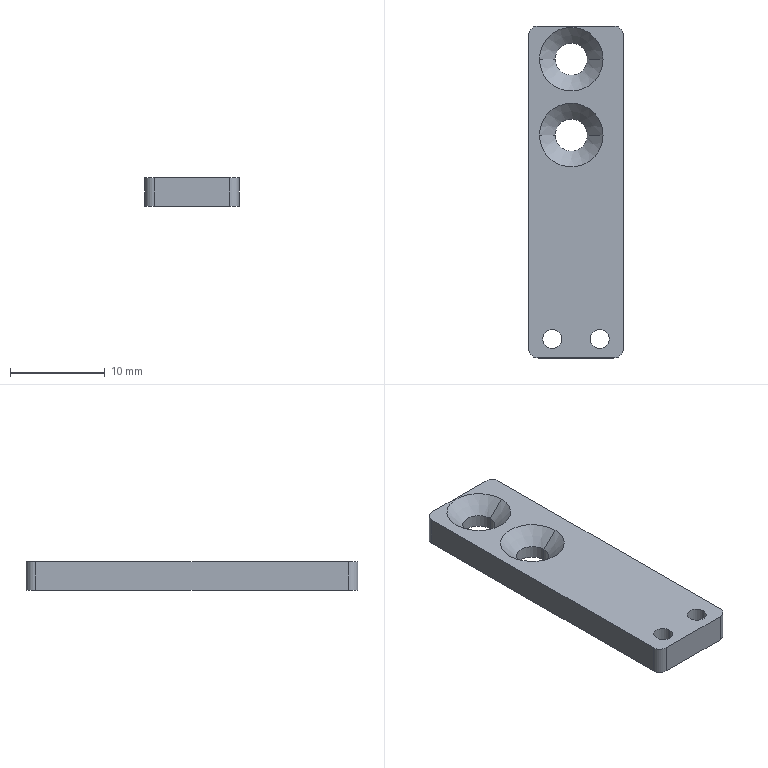Part | STEP file | 11-FG-B08211 | 1 solid | 22 faces | box 10 x 35 x 3 mm | volume 935.086 mm3 | cylinder 12 | plane 6 | cone 4 | commonest cylinder face diameters 2 x8 3.4 x4
STEP:
#1=CARTESIAN_POINT('',(3.5,-15.5,0.));
#2=VERTEX_POINT('',#1);
#3=CARTESIAN_POINT('',(1.5,-15.5,0.));
#4=VERTEX_POINT('',#3);
#5=CARTESIAN_POINT('',(2.5,-15.5,0.));
#6=DIRECTION('',(0.,0.,-1.));
#7=DIRECTION('',(1.,0.,0.));
#8=AXIS2_PLACEMENT_3D('',#5,#6,#7);
#9=CIRCLE('',#8,1.);
#10=EDGE_CURVE('',#2,#4,#9,.T.);
#11=ORIENTED_EDGE('',*,*,#10,.T.);
#12=CARTESIAN_POINT('',(1.5,-15.5,3.));
#13=VERTEX_POINT('',#12);
#14=CARTESIAN_POINT('',(1.5,-15.5,-7.));
#15=DIRECTION('',(0.,0.,1.));
#16=VECTOR('',#15,1000.);
#17=LINE('',#14,#16);
#18=EDGE_CURVE('',#4,#13,#17,.T.);
#19=ORIENTED_EDGE('',*,*,#18,.T.);
#20=CARTESIAN_POINT('',(3.5,-15.5,3.));
#21=VERTEX_POINT('',#20);
#22=CARTESIAN_POINT('',(2.5,-15.5,3.));
#23=DIRECTION('',(0.,0.,-1.));
#24=DIRECTION('',(-1.,0.,0.));
#25=AXIS2_PLACEMENT_3D('',#22,#23,#24);
#26=CIRCLE('',#25,1.);
#27=EDGE_CURVE('',#21,#13,#26,.T.);
#28=ORIENTED_EDGE('',*,*,#27,.F.);
#29=CARTESIAN_POINT('',(3.5,-15.5,-7.));
#30=DIRECTION('',(0.,0.,1.));
#31=VECTOR('',#30,1000.);
#32=LINE('',#29,#31);
#33=EDGE_CURVE('',#2,#21,#32,.T.);
#34=ORIENTED_EDGE('',*,*,#33,.F.);
#35=EDGE_LOOP('',(#11,#19,#28,#34));
#36=FACE_OUTER_BOUND('',#35,.T.);
#37=CARTESIAN_POINT('',(2.5,-15.5,-7.));
#38=DIRECTION('',(0.,0.,1.));
#39=DIRECTION('',(1.,0.,0.));
#40=AXIS2_PLACEMENT_3D('',#37,#38,#39);
#41=CYLINDRICAL_SURFACE('',#40,1.);
#42=ADVANCED_FACE('',(#36),#41,.F.);
#43=CARTESIAN_POINT('',(-3.5,-15.5,0.));
#44=VERTEX_POINT('',#43);
#45=CARTESIAN_POINT('',(-1.5,-15.5,0.));
#46=VERTEX_POINT('',#45);
#47=CARTESIAN_POINT('',(-2.5,-15.5,0.));
#48=DIRECTION('',(0.,0.,1.));
#49=DIRECTION('',(1.,0.,0.));
#50=AXIS2_PLACEMENT_3D('',#47,#48,#49);
#51=CIRCLE('',#50,1.);
#52=EDGE_CURVE('',#44,#46,#51,.T.);
#53=ORIENTED_EDGE('',*,*,#52,.F.);
#54=CARTESIAN_POINT('',(-3.5,-15.5,3.));
#55=VERTEX_POINT('',#54);
#56=CARTESIAN_POINT('',(-3.5,-15.5,-7.));
#57=DIRECTION('',(0.,0.,1.));
#58=VECTOR('',#57,1000.);
#59=LINE('',#56,#58);
#60=EDGE_CURVE('',#44,#55,#59,.T.);
#61=ORIENTED_EDGE('',*,*,#60,.T.);
#62=CARTESIAN_POINT('',(-1.5,-15.5,3.));
#63=VERTEX_POINT('',#62);
#64=CARTESIAN_POINT('',(-2.5,-15.5,3.));
#65=DIRECTION('',(0.,0.,1.));
#66=DIRECTION('',(1.,0.,0.));
#67=AXIS2_PLACEMENT_3D('',#64,#65,#66);
#68=CIRCLE('',#67,1.);
#69=EDGE_CURVE('',#55,#63,#68,.T.);
#70=ORIENTED_EDGE('',*,*,#69,.T.);
#71=CARTESIAN_POINT('',(-1.5,-15.5,-7.));
#72=DIRECTION('',(0.,0.,1.));
#73=VECTOR('',#72,1000.);
#74=LINE('',#71,#73);
#75=EDGE_CURVE('',#46,#63,#74,.T.);
#76=ORIENTED_EDGE('',*,*,#75,.F.);
#77=EDGE_LOOP('',(#53,#61,#70,#76));
#78=FACE_OUTER_BOUND('',#77,.T.);
#79=CARTESIAN_POINT('',(-2.5,-15.5,-7.));
#80=DIRECTION('',(0.,0.,1.));
#81=DIRECTION('',(1.,0.,0.));
#82=AXIS2_PLACEMENT_3D('',#79,#80,#81);
#83=CYLINDRICAL_SURFACE('',#82,1.);
#84=ADVANCED_FACE('',(#78),#83,.F.);
#85=CARTESIAN_POINT('',(-2.2,14.,1.34));
#86=VERTEX_POINT('',#85);
#87=CARTESIAN_POINT('',(1.2,14.,1.34));
#88=VERTEX_POINT('',#87);
#89=CARTESIAN_POINT('',(-0.5,14.,1.34));
#90=DIRECTION('',(0.,0.,1.));
#91=DIRECTION('',(1.,0.,0.));
#92=AXIS2_PLACEMENT_3D('',#89,#90,#91);
#93=CIRCLE('',#92,1.7);
#94=EDGE_CURVE('',#86,#88,#93,.T.);
#95=ORIENTED_EDGE('',*,*,#94,.F.);
#96=CARTESIAN_POINT('',(-3.86,14.,3.));
#97=VERTEX_POINT('',#96);
#98=CARTESIAN_POINT('',(-3.86,14.,3.));
#99=DIRECTION('',(-0.7071,0.,0.7071));
#100=VECTOR('',#99,1000.);
#101=LINE('',#98,#100);
#102=EDGE_CURVE('',#86,#97,#101,.T.);
#103=ORIENTED_EDGE('',*,*,#102,.T.);
#104=CARTESIAN_POINT('',(2.86,14.,3.));
#105=VERTEX_POINT('',#104);
#106=CARTESIAN_POINT('',(-0.5,14.,3.));
#107=DIRECTION('',(0.,0.,1.));
#108=DIRECTION('',(1.,0.,0.));
#109=AXIS2_PLACEMENT_3D('',#106,#107,#108);
#110=CIRCLE('',#109,3.36);
#111=EDGE_CURVE('',#97,#105,#110,.T.);
#112=ORIENTED_EDGE('',*,*,#111,.T.);
#113=CARTESIAN_POINT('',(2.86,14.,3.));
#114=DIRECTION('',(0.7071,0.,0.7071));
#115=VECTOR('',#114,1000.);
#116=LINE('',#113,#115);
#117=EDGE_CURVE('',#88,#105,#116,.T.);
#118=ORIENTED_EDGE('',*,*,#117,.F.);
#119=EDGE_LOOP('',(#95,#103,#112,#118));
#120=FACE_OUTER_BOUND('',#119,.T.);
#121=CARTESIAN_POINT('',(-0.5,14.,3.));
#122=DIRECTION('',(0.,0.,1.));
#123=DIRECTION('',(1.,0.,0.));
#124=AXIS2_PLACEMENT_3D('',#121,#122,#123);
#125=CONICAL_SURFACE('',#124,3.36,0.7854);
#126=ADVANCED_FACE('',(#120),#125,.F.);
#127=CARTESIAN_POINT('',(-2.2,14.,0.));
#128=VERTEX_POINT('',#127);
#129=CARTESIAN_POINT('',(1.2,14.,0.));
#130=VERTEX_POINT('',#129);
#131=CARTESIAN_POINT('',(-0.5,14.,0.));
#132=DIRECTION('',(0.,0.,1.));
#133=DIRECTION('',(1.,0.,0.));
#134=AXIS2_PLACEMENT_3D('',#131,#132,#133);
#135=CIRCLE('',#134,1.7);
#136=EDGE_CURVE('',#128,#130,#135,.T.);
#137=ORIENTED_EDGE('',*,*,#136,.F.);
#138=CARTESIAN_POINT('',(-2.2,14.,3.));
#139=DIRECTION('',(0.,0.,1.));
#140=VECTOR('',#139,1000.);
#141=LINE('',#138,#140);
#142=EDGE_CURVE('',#128,#86,#141,.T.);
#143=ORIENTED_EDGE('',*,*,#142,.T.);
#144=ORIENTED_EDGE('',*,*,#94,.T.);
#145=CARTESIAN_POINT('',(1.2,14.,3.));
#146=DIRECTION('',(0.,0.,1.));
#147=VECTOR('',#146,1000.);
#148=LINE('',#145,#147);
#149=EDGE_CURVE('',#130,#88,#148,.T.);
#150=ORIENTED_EDGE('',*,*,#149,.F.);
#151=EDGE_LOOP('',(#137,#143,#144,#150));
#152=FACE_OUTER_BOUND('',#151,.T.);
#153=CARTESIAN_POINT('',(-0.5,14.,3.));
#154=DIRECTION('',(0.,0.,1.));
#155=DIRECTION('',(1.,0.,0.));
#156=AXIS2_PLACEMENT_3D('',#153,#154,#155);
#157=CYLINDRICAL_SURFACE('',#156,1.7);
#158=ADVANCED_FACE('',(#152),#157,.F.);
#159=CARTESIAN_POINT('',(-2.2,6.,1.34));
#160=VERTEX_POINT('',#159);
#161=CARTESIAN_POINT('',(1.2,6.,1.34));
#162=VERTEX_POINT('',#161);
#163=CARTESIAN_POINT('',(-0.5,6.,1.34));
#164=DIRECTION('',(0.,0.,1.));
#165=DIRECTION('',(1.,0.,0.));
#166=AXIS2_PLACEMENT_3D('',#163,#164,#165);
#167=CIRCLE('',#166,1.7);
#168=EDGE_CURVE('',#160,#162,#167,.T.);
#169=ORIENTED_EDGE('',*,*,#168,.F.);
#170=CARTESIAN_POINT('',(-3.86,6.,3.));
#171=VERTEX_POINT('',#170);
#172=CARTESIAN_POINT('',(-3.86,6.,3.));
#173=DIRECTION('',(-0.7071,0.,0.7071));
#174=VECTOR('',#173,1000.);
#175=LINE('',#172,#174);
#176=EDGE_CURVE('',#160,#171,#175,.T.);
#177=ORIENTED_EDGE('',*,*,#176,.T.);
#178=CARTESIAN_POINT('',(2.86,6.,3.));
#179=VERTEX_POINT('',#178);
#180=CARTESIAN_POINT('',(-0.5,6.,3.));
#181=DIRECTION('',(0.,0.,1.));
#182=DIRECTION('',(1.,0.,0.));
#183=AXIS2_PLACEMENT_3D('',#180,#181,#182);
#184=CIRCLE('',#183,3.36);
#185=EDGE_CURVE('',#171,#179,#184,.T.);
#186=ORIENTED_EDGE('',*,*,#185,.T.);
#187=CARTESIAN_POINT('',(2.86,6.,3.));
#188=DIRECTION('',(0.7071,0.,0.7071));
#189=VECTOR('',#188,1000.);
#190=LINE('',#187,#189);
#191=EDGE_CURVE('',#162,#179,#190,.T.);
#192=ORIENTED_EDGE('',*,*,#191,.F.);
#193=EDGE_LOOP('',(#169,#177,#186,#192));
#194=FACE_OUTER_BOUND('',#193,.T.);
#195=CARTESIAN_POINT('',(-0.5,6.,3.));
#196=DIRECTION('',(0.,0.,1.));
#197=DIRECTION('',(1.,0.,0.));
#198=AXIS2_PLACEMENT_3D('',#195,#196,#197);
#199=CONICAL_SURFACE('',#198,3.36,0.7854);
#200=ADVANCED_FACE('',(#194),#199,.F.);
#201=CARTESIAN_POINT('',(-2.2,6.,0.));
#202=VERTEX_POINT('',#201);
#203=CARTESIAN_POINT('',(1.2,6.,0.));
#204=VERTEX_POINT('',#203);
#205=CARTESIAN_POINT('',(-0.5,6.,0.));
#206=DIRECTION('',(0.,0.,1.));
#207=DIRECTION('',(1.,0.,0.));
#208=AXIS2_PLACEMENT_3D('',#205,#206,#207);
#209=CIRCLE('',#208,1.7);
#210=EDGE_CURVE('',#202,#204,#209,.T.);
#211=ORIENTED_EDGE('',*,*,#210,.F.);
#212=CARTESIAN_POINT('',(-2.2,6.,3.));
#213=DIRECTION('',(0.,0.,1.));
#214=VECTOR('',#213,1000.);
#215=LINE('',#212,#214);
#216=EDGE_CURVE('',#202,#160,#215,.T.);
#217=ORIENTED_EDGE('',*,*,#216,.T.);
#218=ORIENTED_EDGE('',*,*,#168,.T.);
#219=CARTESIAN_POINT('',(1.2,6.,3.));
#220=DIRECTION('',(0.,0.,1.));
#221=VECTOR('',#220,1000.);
#222=LINE('',#219,#221);
#223=EDGE_CURVE('',#204,#162,#222,.T.);
#224=ORIENTED_EDGE('',*,*,#223,.F.);
#225=EDGE_LOOP('',(#211,#217,#218,#224));
#226=FACE_OUTER_BOUND('',#225,.T.);
#227=CARTESIAN_POINT('',(-0.5,6.,3.));
#228=DIRECTION('',(0.,0.,1.));
#229=DIRECTION('',(1.,0.,0.));
#230=AXIS2_PLACEMENT_3D('',#227,#228,#229);
#231=CYLINDRICAL_SURFACE('',#230,1.7);
#232=ADVANCED_FACE('',(#226),#231,.F.);
#233=CARTESIAN_POINT('',(5.,-16.5,0.));
#234=VERTEX_POINT('',#233);
#235=CARTESIAN_POINT('',(5.,16.5,0.));
#236=VERTEX_POINT('',#235);
#237=CARTESIAN_POINT('',(5.,17.5,0.));
#238=DIRECTION('',(0.,1.,0.));
#239=VECTOR('',#238,1000.);
#240=LINE('',#237,#239);
#241=EDGE_CURVE('',#234,#236,#240,.T.);
#242=ORIENTED_EDGE('',*,*,#241,.T.);
#243=CARTESIAN_POINT('',(5.,16.5,3.));
#244=VERTEX_POINT('',#243);
#245=CARTESIAN_POINT('',(5.,16.5,3.));
#246=DIRECTION('',(0.,0.,1.));
#247=VECTOR('',#246,1000.);
#248=LINE('',#245,#247);
#249=EDGE_CURVE('',#236,#244,#248,.T.);
#250=ORIENTED_EDGE('',*,*,#249,.T.);
#251=CARTESIAN_POINT('',(5.,-16.5,3.));
#252=VERTEX_POINT('',#251);
#253=CARTESIAN_POINT('',(5.,17.5,3.));
#254=DIRECTION('',(0.,1.,0.));
#255=VECTOR('',#254,1000.);
#256=LINE('',#253,#255);
#257=EDGE_CURVE('',#252,#244,#256,.T.);
#258=ORIENTED_EDGE('',*,*,#257,.F.);
#259=CARTESIAN_POINT('',(5.,-16.5,3.));
#260=DIRECTION('',(0.,0.,-1.));
#261=VECTOR('',#260,1000.);
#262=LINE('',#259,#261);
#263=EDGE_CURVE('',#252,#234,#262,.T.);
#264=ORIENTED_EDGE('',*,*,#263,.T.);
#265=EDGE_LOOP('',(#242,#250,#258,#264));
#266=FACE_OUTER_BOUND('',#265,.T.);
#267=CARTESIAN_POINT('',(5.,17.5,3.));
#268=DIRECTION('',(-1.,0.,0.));
#269=DIRECTION('',(0.,-1.,0.));
#270=AXIS2_PLACEMENT_3D('',#267,#268,#269);
#271=PLANE('',#270);
#272=ADVANCED_FACE('',(#266),#271,.F.);
#273=CARTESIAN_POINT('',(4.,17.5,3.));
#274=VERTEX_POINT('',#273);
#275=CARTESIAN_POINT('',(-4.,17.5,3.));
#276=VERTEX_POINT('',#275);
#277=CARTESIAN_POINT('',(-5.,17.5,3.));
#278=DIRECTION('',(-1.,0.,0.));
#279=VECTOR('',#278,1000.);
#280=LINE('',#277,#279);
#281=EDGE_CURVE('',#274,#276,#280,.T.);
#282=ORIENTED_EDGE('',*,*,#281,.F.);
#283=CARTESIAN_POINT('',(4.,17.5,0.));
#284=VERTEX_POINT('',#283);
#285=CARTESIAN_POINT('',(4.,17.5,3.));
#286=DIRECTION('',(0.,0.,-1.));
#287=VECTOR('',#286,1000.);
#288=LINE('',#285,#287);
#289=EDGE_CURVE('',#274,#284,#288,.T.);
#290=ORIENTED_EDGE('',*,*,#289,.T.);
#291=CARTESIAN_POINT('',(-4.,17.5,0.));
#292=VERTEX_POINT('',#291);
#293=CARTESIAN_POINT('',(-5.,17.5,0.));
#294=DIRECTION('',(-1.,0.,0.));
#295=VECTOR('',#294,1000.);
#296=LINE('',#293,#295);
#297=EDGE_CURVE('',#284,#292,#296,.T.);
#298=ORIENTED_EDGE('',*,*,#297,.T.);
#299=CARTESIAN_POINT('',(-4.,17.5,3.));
#300=DIRECTION('',(0.,0.,1.));
#301=VECTOR('',#300,1000.);
#302=LINE('',#299,#301);
#303=EDGE_CURVE('',#292,#276,#302,.T.);
#304=ORIENTED_EDGE('',*,*,#303,.T.);
#305=EDGE_LOOP('',(#282,#290,#298,#304));
#306=FACE_OUTER_BOUND('',#305,.T.);
#307=CARTESIAN_POINT('',(-5.,17.5,3.));
#308=DIRECTION('',(0.,-1.,0.));
#309=DIRECTION('',(0.,0.,-1.));
#310=AXIS2_PLACEMENT_3D('',#307,#308,#309);
#311=PLANE('',#310);
#312=ADVANCED_FACE('',(#306),#311,.F.);
#313=CARTESIAN_POINT('',(-5.,16.5,3.));
#314=VERTEX_POINT('',#313);
#315=CARTESIAN_POINT('',(-5.,-16.5,3.));
#316=VERTEX_POINT('',#315);
#317=CARTESIAN_POINT('',(-5.,17.5,3.));
#318=DIRECTION('',(0.,-1.,0.));
#319=VECTOR('',#318,1000.);
#320=LINE('',#317,#319);
#321=EDGE_CURVE('',#314,#316,#320,.T.);
#322=ORIENTED_EDGE('',*,*,#321,.F.);
#323=CARTESIAN_POINT('',(-5.,16.5,0.));
#324=VERTEX_POINT('',#323);
#325=CARTESIAN_POINT('',(-5.,16.5,3.));
#326=DIRECTION('',(0.,0.,-1.));
#327=VECTOR('',#326,1000.);
#328=LINE('',#325,#327);
#329=EDGE_CURVE('',#314,#324,#328,.T.);
#330=ORIENTED_EDGE('',*,*,#329,.T.);
#331=CARTESIAN_POINT('',(-5.,-16.5,0.));
#332=VERTEX_POINT('',#331);
#333=CARTESIAN_POINT('',(-5.,17.5,0.));
#334=DIRECTION('',(0.,-1.,0.));
#335=VECTOR('',#334,1000.);
#336=LINE('',#333,#335);
#337=EDGE_CURVE('',#324,#332,#336,.T.);
#338=ORIENTED_EDGE('',*,*,#337,.T.);
#339=CARTESIAN_POINT('',(-5.,-16.5,3.));
#340=DIRECTION('',(0.,0.,1.));
#341=VECTOR('',#340,1000.);
#342=LINE('',#339,#341);
#343=EDGE_CURVE('',#332,#316,#342,.T.);
#344=ORIENTED_EDGE('',*,*,#343,.T.);
#345=EDGE_LOOP('',(#322,#330,#338,#344));
#346=FACE_OUTER_BOUND('',#345,.T.);
#347=CARTESIAN_POINT('',(-5.,17.5,3.));
#348=DIRECTION('',(1.,0.,0.));
#349=DIRECTION('',(0.,1.,0.));
#350=AXIS2_PLACEMENT_3D('',#347,#348,#349);
#351=PLANE('',#350);
#352=ADVANCED_FACE('',(#346),#351,.F.);
#353=CARTESIAN_POINT('',(-4.,-17.5,0.));
#354=VERTEX_POINT('',#353);
#355=CARTESIAN_POINT('',(4.,-17.5,0.));
#356=VERTEX_POINT('',#355);
#357=CARTESIAN_POINT('',(-5.,-17.5,0.));
#358=DIRECTION('',(1.,0.,0.));
#359=VECTOR('',#358,1000.);
#360=LINE('',#357,#359);
#361=EDGE_CURVE('',#354,#356,#360,.T.);
#362=ORIENTED_EDGE('',*,*,#361,.T.);
#363=CARTESIAN_POINT('',(4.,-17.5,3.));
#364=VERTEX_POINT('',#363);
#365=CARTESIAN_POINT('',(4.,-17.5,3.));
#366=DIRECTION('',(0.,0.,1.));
#367=VECTOR('',#366,1000.);
#368=LINE('',#365,#367);
#369=EDGE_CURVE('',#356,#364,#368,.T.);
#370=ORIENTED_EDGE('',*,*,#369,.T.);
#371=CARTESIAN_POINT('',(-4.,-17.5,3.));
#372=VERTEX_POINT('',#371);
#373=CARTESIAN_POINT('',(-5.,-17.5,3.));
#374=DIRECTION('',(1.,0.,0.));
#375=VECTOR('',#374,1000.);
#376=LINE('',#373,#375);
#377=EDGE_CURVE('',#372,#364,#376,.T.);
#378=ORIENTED_EDGE('',*,*,#377,.F.);
#379=CARTESIAN_POINT('',(-4.,-17.5,3.));
#380=DIRECTION('',(0.,0.,-1.));
#381=VECTOR('',#380,1000.);
#382=LINE('',#379,#381);
#383=EDGE_CURVE('',#372,#354,#382,.T.);
#384=ORIENTED_EDGE('',*,*,#383,.T.);
#385=EDGE_LOOP('',(#362,#370,#378,#384));
#386=FACE_OUTER_BOUND('',#385,.T.);
#387=CARTESIAN_POINT('',(-5.,-17.5,3.));
#388=DIRECTION('',(0.,1.,0.));
#389=DIRECTION('',(0.,0.,1.));
#390=AXIS2_PLACEMENT_3D('',#387,#388,#389);
#391=PLANE('',#390);
#392=ADVANCED_FACE('',(#386),#391,.F.);
#393=ORIENTED_EDGE('',*,*,#27,.T.);
#394=CARTESIAN_POINT('',(2.5,-15.5,3.));
#395=DIRECTION('',(0.,0.,-1.));
#396=DIRECTION('',(-1.,0.,0.));
#397=AXIS2_PLACEMENT_3D('',#394,#395,#396);
#398=CIRCLE('',#397,1.);
#399=EDGE_CURVE('',#13,#21,#398,.T.);
#400=ORIENTED_EDGE('',*,*,#399,.T.);
#401=EDGE_LOOP('',(#393,#400));
#402=FACE_BOUND('',#401,.T.);
#403=CARTESIAN_POINT('',(-2.5,-15.5,3.));
#404=DIRECTION('',(0.,0.,1.));
#405=DIRECTION('',(1.,0.,0.));
#406=AXIS2_PLACEMENT_3D('',#403,#404,#405);
#407=CIRCLE('',#406,1.);
#408=EDGE_CURVE('',#63,#55,#407,.T.);
#409=ORIENTED_EDGE('',*,*,#408,.F.);
#410=ORIENTED_EDGE('',*,*,#69,.F.);
#411=EDGE_LOOP('',(#409,#410));
#412=FACE_BOUND('',#411,.T.);
#413=CARTESIAN_POINT('',(-0.5,14.,3.));
#414=DIRECTION('',(0.,0.,1.));
#415=DIRECTION('',(1.,0.,0.));
#416=AXIS2_PLACEMENT_3D('',#413,#414,#415);
#417=CIRCLE('',#416,3.36);
#418=EDGE_CURVE('',#105,#97,#417,.T.);
#419=ORIENTED_EDGE('',*,*,#418,.F.);
#420=ORIENTED_EDGE('',*,*,#111,.F.);
#421=EDGE_LOOP('',(#419,#420));
#422=FACE_BOUND('',#421,.T.);
#423=CARTESIAN_POINT('',(-0.5,6.,3.));
#424=DIRECTION('',(0.,0.,1.));
#425=DIRECTION('',(1.,0.,0.));
#426=AXIS2_PLACEMENT_3D('',#423,#424,#425);
#427=CIRCLE('',#426,3.36);
#428=EDGE_CURVE('',#179,#171,#427,.T.);
#429=ORIENTED_EDGE('',*,*,#428,.F.);
#430=ORIENTED_EDGE('',*,*,#185,.F.);
#431=EDGE_LOOP('',(#429,#430));
#432=FACE_BOUND('',#431,.T.);
#433=ORIENTED_EDGE('',*,*,#257,.T.);
#434=CARTESIAN_POINT('',(4.,16.5,3.));
#435=DIRECTION('',(0.,0.,1.));
#436=DIRECTION('',(1.,0.,0.));
#437=AXIS2_PLACEMENT_3D('',#434,#435,#436);
#438=CIRCLE('',#437,1.);
#439=EDGE_CURVE('',#244,#274,#438,.T.);
#440=ORIENTED_EDGE('',*,*,#439,.T.);
#441=ORIENTED_EDGE('',*,*,#281,.T.);
#442=CARTESIAN_POINT('',(-4.,16.5,3.));
#443=DIRECTION('',(0.,0.,1.));
#444=DIRECTION('',(1.,0.,0.));
#445=AXIS2_PLACEMENT_3D('',#442,#443,#444);
#446=CIRCLE('',#445,1.);
#447=EDGE_CURVE('',#276,#314,#446,.T.);
#448=ORIENTED_EDGE('',*,*,#447,.T.);
#449=ORIENTED_EDGE('',*,*,#321,.T.);
#450=CARTESIAN_POINT('',(-4.,-16.5,3.));
#451=DIRECTION('',(0.,0.,1.));
#452=DIRECTION('',(1.,0.,0.));
#453=AXIS2_PLACEMENT_3D('',#450,#451,#452);
#454=CIRCLE('',#453,1.);
#455=EDGE_CURVE('',#316,#372,#454,.T.);
#456=ORIENTED_EDGE('',*,*,#455,.T.);
#457=ORIENTED_EDGE('',*,*,#377,.T.);
#458=CARTESIAN_POINT('',(4.,-16.5,3.));
#459=DIRECTION('',(0.,0.,1.));
#460=DIRECTION('',(1.,0.,0.));
#461=AXIS2_PLACEMENT_3D('',#458,#459,#460);
#462=CIRCLE('',#461,1.);
#463=EDGE_CURVE('',#364,#252,#462,.T.);
#464=ORIENTED_EDGE('',*,*,#463,.T.);
#465=EDGE_LOOP('',(#433,#440,#441,#448,#449,#456,#457,#464));
#466=FACE_OUTER_BOUND('',#465,.T.);
#467=CARTESIAN_POINT('',(0.,0.,3.));
#468=DIRECTION('',(0.,0.,1.));
#469=DIRECTION('',(1.,0.,0.));
#470=AXIS2_PLACEMENT_3D('',#467,#468,#469);
#471=PLANE('',#470);
#472=ADVANCED_FACE('',(#402,#412,#422,#432,#466),#471,.T.);
#473=ORIENTED_EDGE('',*,*,#10,.F.);
#474=CARTESIAN_POINT('',(2.5,-15.5,0.));
#475=DIRECTION('',(0.,0.,-1.));
#476=DIRECTION('',(1.,0.,0.));
#477=AXIS2_PLACEMENT_3D('',#474,#475,#476);
#478=CIRCLE('',#477,1.);
#479=EDGE_CURVE('',#4,#2,#478,.T.);
#480=ORIENTED_EDGE('',*,*,#479,.F.);
#481=EDGE_LOOP('',(#473,#480));
#482=FACE_BOUND('',#481,.T.);
#483=CARTESIAN_POINT('',(-2.5,-15.5,0.));
#484=DIRECTION('',(0.,0.,1.));
#485=DIRECTION('',(1.,0.,0.));
#486=AXIS2_PLACEMENT_3D('',#483,#484,#485);
#487=CIRCLE('',#486,1.);
#488=EDGE_CURVE('',#46,#44,#487,.T.);
#489=ORIENTED_EDGE('',*,*,#488,.T.);
#490=ORIENTED_EDGE('',*,*,#52,.T.);
#491=EDGE_LOOP('',(#489,#490));
#492=FACE_BOUND('',#491,.T.);
#493=CARTESIAN_POINT('',(-0.5,14.,0.));
#494=DIRECTION('',(0.,0.,1.));
#495=DIRECTION('',(1.,0.,0.));
#496=AXIS2_PLACEMENT_3D('',#493,#494,#495);
#497=CIRCLE('',#496,1.7);
#498=EDGE_CURVE('',#130,#128,#497,.T.);
#499=ORIENTED_EDGE('',*,*,#498,.T.);
#500=ORIENTED_EDGE('',*,*,#136,.T.);
#501=EDGE_LOOP('',(#499,#500));
#502=FACE_BOUND('',#501,.T.);
#503=CARTESIAN_POINT('',(-0.5,6.,0.));
#504=DIRECTION('',(0.,0.,1.));
#505=DIRECTION('',(1.,0.,0.));
#506=AXIS2_PLACEMENT_3D('',#503,#504,#505);
#507=CIRCLE('',#506,1.7);
#508=EDGE_CURVE('',#204,#202,#507,.T.);
#509=ORIENTED_EDGE('',*,*,#508,.T.);
#510=ORIENTED_EDGE('',*,*,#210,.T.);
#511=EDGE_LOOP('',(#509,#510));
#512=FACE_BOUND('',#511,.T.);
#513=ORIENTED_EDGE('',*,*,#297,.F.);
#514=CARTESIAN_POINT('',(4.,16.5,0.));
#515=DIRECTION('',(0.,0.,-1.));
#516=DIRECTION('',(1.,0.,0.));
#517=AXIS2_PLACEMENT_3D('',#514,#515,#516);
#518=CIRCLE('',#517,1.);
#519=EDGE_CURVE('',#284,#236,#518,.T.);
#520=ORIENTED_EDGE('',*,*,#519,.T.);
#521=ORIENTED_EDGE('',*,*,#241,.F.);
#522=CARTESIAN_POINT('',(4.,-16.5,0.));
#523=DIRECTION('',(0.,0.,-1.));
#524=DIRECTION('',(1.,0.,0.));
#525=AXIS2_PLACEMENT_3D('',#522,#523,#524);
#526=CIRCLE('',#525,1.);
#527=EDGE_CURVE('',#234,#356,#526,.T.);
#528=ORIENTED_EDGE('',*,*,#527,.T.);
#529=ORIENTED_EDGE('',*,*,#361,.F.);
#530=CARTESIAN_POINT('',(-4.,-16.5,0.));
#531=DIRECTION('',(0.,0.,-1.));
#532=DIRECTION('',(1.,0.,0.));
#533=AXIS2_PLACEMENT_3D('',#530,#531,#532);
#534=CIRCLE('',#533,1.);
#535=EDGE_CURVE('',#354,#332,#534,.T.);
#536=ORIENTED_EDGE('',*,*,#535,.T.);
#537=ORIENTED_EDGE('',*,*,#337,.F.);
#538=CARTESIAN_POINT('',(-4.,16.5,0.));
#539=DIRECTION('',(0.,0.,-1.));
#540=DIRECTION('',(1.,0.,0.));
#541=AXIS2_PLACEMENT_3D('',#538,#539,#540);
#542=CIRCLE('',#541,1.);
#543=EDGE_CURVE('',#324,#292,#542,.T.);
#544=ORIENTED_EDGE('',*,*,#543,.T.);
#545=EDGE_LOOP('',(#513,#520,#521,#528,#529,#536,#537,#544));
#546=FACE_OUTER_BOUND('',#545,.T.);
#547=CARTESIAN_POINT('',(0.,0.,0.));
#548=DIRECTION('',(0.,0.,1.));
#549=DIRECTION('',(1.,0.,0.));
#550=AXIS2_PLACEMENT_3D('',#547,#548,#549);
#551=PLANE('',#550);
#552=ADVANCED_FACE('',(#482,#492,#502,#512,#546),#551,.F.);
#553=ORIENTED_EDGE('',*,*,#216,.F.);
#554=ORIENTED_EDGE('',*,*,#508,.F.);
#555=ORIENTED_EDGE('',*,*,#223,.T.);
#556=CARTESIAN_POINT('',(-0.5,6.,1.34));
#557=DIRECTION('',(0.,0.,1.));
#558=DIRECTION('',(1.,0.,0.));
#559=AXIS2_PLACEMENT_3D('',#556,#557,#558);
#560=CIRCLE('',#559,1.7);
#561=EDGE_CURVE('',#162,#160,#560,.T.);
#562=ORIENTED_EDGE('',*,*,#561,.T.);
#563=EDGE_LOOP('',(#553,#554,#555,#562));
#564=FACE_OUTER_BOUND('',#563,.T.);
#565=CARTESIAN_POINT('',(-0.5,6.,3.));
#566=DIRECTION('',(0.,0.,1.));
#567=DIRECTION('',(1.,0.,0.));
#568=AXIS2_PLACEMENT_3D('',#565,#566,#567);
#569=CYLINDRICAL_SURFACE('',#568,1.7);
#570=ADVANCED_FACE('',(#564),#569,.F.);
#571=ORIENTED_EDGE('',*,*,#176,.F.);
#572=ORIENTED_EDGE('',*,*,#561,.F.);
#573=ORIENTED_EDGE('',*,*,#191,.T.);
#574=ORIENTED_EDGE('',*,*,#428,.T.);
#575=EDGE_LOOP('',(#571,#572,#573,#574));
#576=FACE_OUTER_BOUND('',#575,.T.);
#577=CARTESIAN_POINT('',(-0.5,6.,3.));
#578=DIRECTION('',(0.,0.,1.));
#579=DIRECTION('',(1.,0.,0.));
#580=AXIS2_PLACEMENT_3D('',#577,#578,#579);
#581=CONICAL_SURFACE('',#580,3.36,0.7854);
#582=ADVANCED_FACE('',(#576),#581,.F.);
#583=ORIENTED_EDGE('',*,*,#142,.F.);
#584=ORIENTED_EDGE('',*,*,#498,.F.);
#585=ORIENTED_EDGE('',*,*,#149,.T.);
#586=CARTESIAN_POINT('',(-0.5,14.,1.34));
#587=DIRECTION('',(0.,0.,1.));
#588=DIRECTION('',(1.,0.,0.));
#589=AXIS2_PLACEMENT_3D('',#586,#587,#588);
#590=CIRCLE('',#589,1.7);
#591=EDGE_CURVE('',#88,#86,#590,.T.);
#592=ORIENTED_EDGE('',*,*,#591,.T.);
#593=EDGE_LOOP('',(#583,#584,#585,#592));
#594=FACE_OUTER_BOUND('',#593,.T.);
#595=CARTESIAN_POINT('',(-0.5,14.,3.));
#596=DIRECTION('',(0.,0.,1.));
#597=DIRECTION('',(1.,0.,0.));
#598=AXIS2_PLACEMENT_3D('',#595,#596,#597);
#599=CYLINDRICAL_SURFACE('',#598,1.7);
#600=ADVANCED_FACE('',(#594),#599,.F.);
#601=ORIENTED_EDGE('',*,*,#102,.F.);
#602=ORIENTED_EDGE('',*,*,#591,.F.);
#603=ORIENTED_EDGE('',*,*,#117,.T.);
#604=ORIENTED_EDGE('',*,*,#418,.T.);
#605=EDGE_LOOP('',(#601,#602,#603,#604));
#606=FACE_OUTER_BOUND('',#605,.T.);
#607=CARTESIAN_POINT('',(-0.5,14.,3.));
#608=DIRECTION('',(0.,0.,1.));
#609=DIRECTION('',(1.,0.,0.));
#610=AXIS2_PLACEMENT_3D('',#607,#608,#609);
#611=CONICAL_SURFACE('',#610,3.36,0.7854);
#612=ADVANCED_FACE('',(#606),#611,.F.);
#613=ORIENTED_EDGE('',*,*,#439,.F.);
#614=ORIENTED_EDGE('',*,*,#249,.F.);
#615=ORIENTED_EDGE('',*,*,#519,.F.);
#616=ORIENTED_EDGE('',*,*,#289,.F.);
#617=EDGE_LOOP('',(#613,#614,#615,#616));
#618=FACE_OUTER_BOUND('',#617,.T.);
#619=CARTESIAN_POINT('',(4.,16.5,3.));
#620=DIRECTION('',(0.,0.,-1.));
#621=DIRECTION('',(-1.,0.,0.));
#622=AXIS2_PLACEMENT_3D('',#619,#620,#621);
#623=CYLINDRICAL_SURFACE('',#622,1.);
#624=ADVANCED_FACE('',(#618),#623,.T.);
#625=ORIENTED_EDGE('',*,*,#447,.F.);
#626=ORIENTED_EDGE('',*,*,#303,.F.);
#627=ORIENTED_EDGE('',*,*,#543,.F.);
#628=ORIENTED_EDGE('',*,*,#329,.F.);
#629=EDGE_LOOP('',(#625,#626,#627,#628));
#630=FACE_OUTER_BOUND('',#629,.T.);
#631=CARTESIAN_POINT('',(-4.,16.5,3.));
#632=DIRECTION('',(0.,0.,-1.));
#633=DIRECTION('',(-1.,0.,0.));
#634=AXIS2_PLACEMENT_3D('',#631,#632,#633);
#635=CYLINDRICAL_SURFACE('',#634,1.);
#636=ADVANCED_FACE('',(#630),#635,.T.);
#637=ORIENTED_EDGE('',*,*,#463,.F.);
#638=ORIENTED_EDGE('',*,*,#369,.F.);
#639=ORIENTED_EDGE('',*,*,#527,.F.);
#640=ORIENTED_EDGE('',*,*,#263,.F.);
#641=EDGE_LOOP('',(#637,#638,#639,#640));
#642=FACE_OUTER_BOUND('',#641,.T.);
#643=CARTESIAN_POINT('',(4.,-16.5,3.));
#644=DIRECTION('',(0.,0.,-1.));
#645=DIRECTION('',(-1.,0.,0.));
#646=AXIS2_PLACEMENT_3D('',#643,#644,#645);
#647=CYLINDRICAL_SURFACE('',#646,1.);
#648=ADVANCED_FACE('',(#642),#647,.T.);
#649=ORIENTED_EDGE('',*,*,#455,.F.);
#650=ORIENTED_EDGE('',*,*,#343,.F.);
#651=ORIENTED_EDGE('',*,*,#535,.F.);
#652=ORIENTED_EDGE('',*,*,#383,.F.);
#653=EDGE_LOOP('',(#649,#650,#651,#652));
#654=FACE_OUTER_BOUND('',#653,.T.);
#655=CARTESIAN_POINT('',(-4.,-16.5,3.));
#656=DIRECTION('',(0.,0.,-1.));
#657=DIRECTION('',(-1.,0.,0.));
#658=AXIS2_PLACEMENT_3D('',#655,#656,#657);
#659=CYLINDRICAL_SURFACE('',#658,1.);
#660=ADVANCED_FACE('',(#654),#659,.T.);
#661=ORIENTED_EDGE('',*,*,#60,.F.);
#662=ORIENTED_EDGE('',*,*,#488,.F.);
#663=ORIENTED_EDGE('',*,*,#75,.T.);
#664=ORIENTED_EDGE('',*,*,#408,.T.);
#665=EDGE_LOOP('',(#661,#662,#663,#664));
#666=FACE_OUTER_BOUND('',#665,.T.);
#667=CARTESIAN_POINT('',(-2.5,-15.5,-7.));
#668=DIRECTION('',(0.,0.,1.));
#669=DIRECTION('',(1.,0.,0.));
#670=AXIS2_PLACEMENT_3D('',#667,#668,#669);
#671=CYLINDRICAL_SURFACE('',#670,1.);
#672=ADVANCED_FACE('',(#666),#671,.F.);
#673=ORIENTED_EDGE('',*,*,#18,.F.);
#674=ORIENTED_EDGE('',*,*,#479,.T.);
#675=ORIENTED_EDGE('',*,*,#33,.T.);
#676=ORIENTED_EDGE('',*,*,#399,.F.);
#677=EDGE_LOOP('',(#673,#674,#675,#676));
#678=FACE_OUTER_BOUND('',#677,.T.);
#679=CARTESIAN_POINT('',(2.5,-15.5,-7.));
#680=DIRECTION('',(0.,0.,1.));
#681=DIRECTION('',(1.,0.,0.));
#682=AXIS2_PLACEMENT_3D('',#679,#680,#681);
#683=CYLINDRICAL_SURFACE('',#682,1.);
#684=ADVANCED_FACE('',(#678),#683,.F.);
#685=CLOSED_SHELL('',(#42,#84,#126,#158,#200,#232,#272,#312,#352,#392,#472,#552,#570,#582,#600,#612,#624,#636,#648,#660,#672,#684));
#686=MANIFOLD_SOLID_BREP('',#685);
#687=CARTESIAN_POINT('',(0.,0.,0.));
#688=DIRECTION('',(0.,0.,1.));
#689=DIRECTION('',(1.,0.,0.));
#690=AXIS2_PLACEMENT_3D('',#687,#688,#689);
#691=(LENGTH_UNIT()NAMED_UNIT(*)SI_UNIT(.MILLI.,.METRE.));
#692=UNCERTAINTY_MEASURE_WITH_UNIT(LENGTH_MEASURE(0.00001),#691,'','');
#693=(NAMED_UNIT(*)PLANE_ANGLE_UNIT()SI_UNIT($,.RADIAN.));
#694=(NAMED_UNIT(*)SI_UNIT($,.STERADIAN.)SOLID_ANGLE_UNIT());
#695=(GEOMETRIC_REPRESENTATION_CONTEXT(3)GLOBAL_UNCERTAINTY_ASSIGNED_CONTEXT((#692))GLOBAL_UNIT_ASSIGNED_CONTEXT((#691,#693,#694))REPRESENTATION_CONTEXT('',''));
#696=ADVANCED_BREP_SHAPE_REPRESENTATION('',(#686,#690),#695);